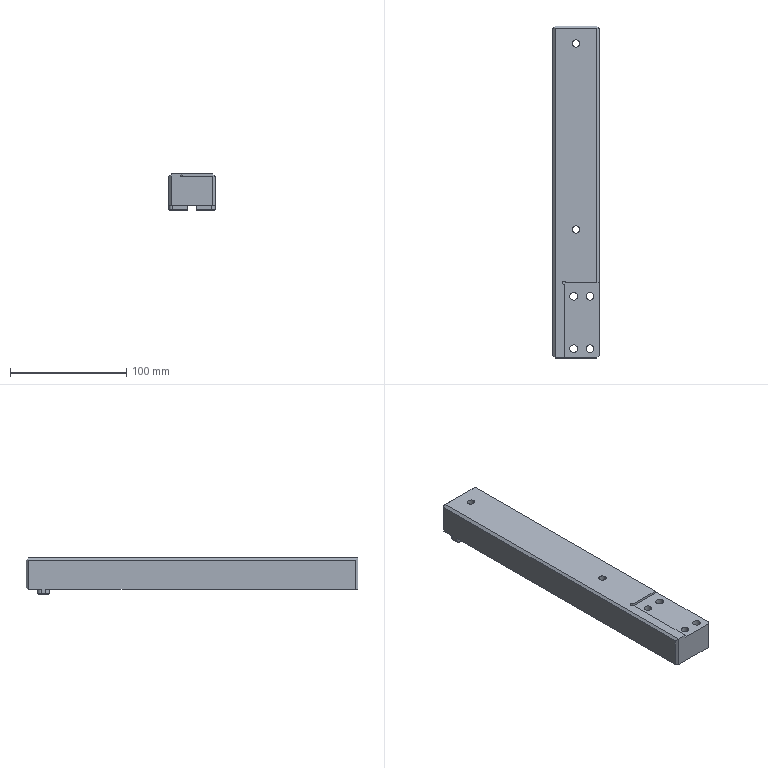Part | STEP file | Screen clamp adjusting plate^Right screen clamp assembly_Screen assembly_PS-3045E-LDJ2 | 1 solid | 66 faces | box 40 x 285.5 x 31 mm | volume 297627 mm3 | plane 37 | cylinder 25 | cone 4 | commonest cylinder face diameters 6.6 x8 11 x8 6 x4 6.2 x4 3 x1